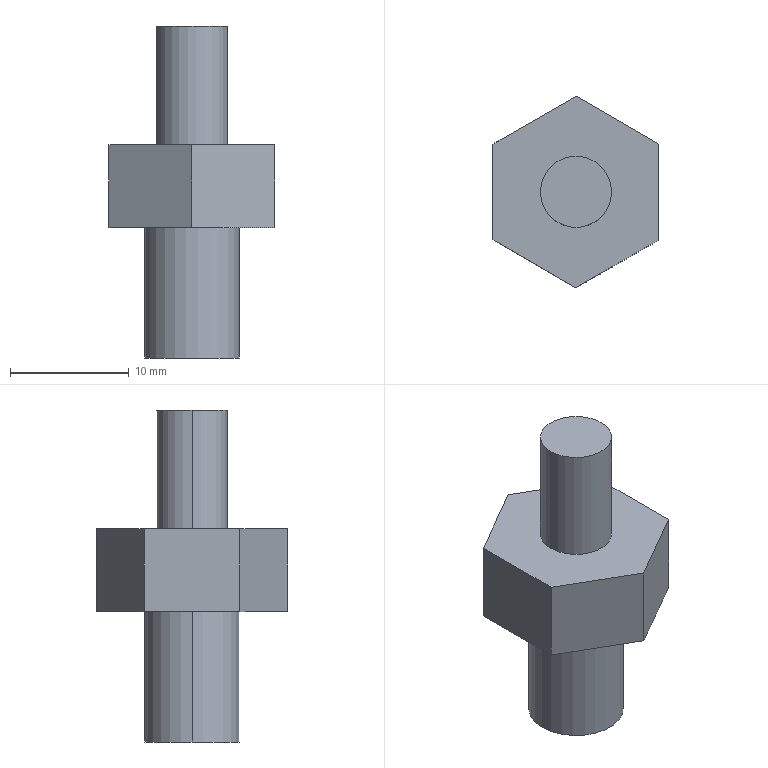Part | STEP file | Connecting bolt | 1 solid | 14 faces | box 14 x 16.166 x 28 mm | volume 2024 mm3 | plane 10 | cylinder 4 | commonest cylinder face diameters 6 x2 8 x2
STEP:
#1=CARTESIAN_POINT('',(-4.,0.,-14.5));
#2=VERTEX_POINT('',#1);
#3=CARTESIAN_POINT('',(4.,0.,-14.5));
#4=VERTEX_POINT('',#3);
#5=CARTESIAN_POINT('',(0.,0.,-14.5));
#6=DIRECTION('',(0.,0.,-1.));
#7=DIRECTION('',(-1.,0.,0.));
#8=AXIS2_PLACEMENT_3D('',#5,#6,#7);
#9=CIRCLE('',#8,4.);
#10=EDGE_CURVE('',#2,#4,#9,.T.);
#11=ORIENTED_EDGE('',*,*,#10,.F.);
#12=CARTESIAN_POINT('',(-4.,0.,-3.5));
#13=VERTEX_POINT('',#12);
#14=CARTESIAN_POINT('',(-4.,0.,-14.5));
#15=DIRECTION('',(0.,0.,1.));
#16=VECTOR('',#15,1000.);
#17=LINE('',#14,#16);
#18=EDGE_CURVE('',#2,#13,#17,.T.);
#19=ORIENTED_EDGE('',*,*,#18,.T.);
#20=CARTESIAN_POINT('',(4.,0.,-3.5));
#21=VERTEX_POINT('',#20);
#22=CARTESIAN_POINT('',(0.,0.,-3.5));
#23=DIRECTION('',(0.,0.,-1.));
#24=DIRECTION('',(1.,0.,0.));
#25=AXIS2_PLACEMENT_3D('',#22,#23,#24);
#26=CIRCLE('',#25,4.);
#27=EDGE_CURVE('',#13,#21,#26,.T.);
#28=ORIENTED_EDGE('',*,*,#27,.T.);
#29=CARTESIAN_POINT('',(4.,0.,-14.5));
#30=DIRECTION('',(0.,0.,1.));
#31=VECTOR('',#30,1000.);
#32=LINE('',#29,#31);
#33=EDGE_CURVE('',#4,#21,#32,.T.);
#34=ORIENTED_EDGE('',*,*,#33,.F.);
#35=EDGE_LOOP('',(#11,#19,#28,#34));
#36=FACE_OUTER_BOUND('',#35,.T.);
#37=CARTESIAN_POINT('',(0.,0.,-14.5));
#38=DIRECTION('',(0.,0.,1.));
#39=DIRECTION('',(1.,0.,0.));
#40=AXIS2_PLACEMENT_3D('',#37,#38,#39);
#41=CYLINDRICAL_SURFACE('',#40,4.);
#42=ADVANCED_FACE('',(#36),#41,.T.);
#43=CARTESIAN_POINT('',(3.,0.,13.5));
#44=VERTEX_POINT('',#43);
#45=CARTESIAN_POINT('',(-3.,0.,13.5));
#46=VERTEX_POINT('',#45);
#47=CARTESIAN_POINT('',(0.,0.,13.5));
#48=DIRECTION('',(0.,0.,1.));
#49=DIRECTION('',(1.,0.,0.));
#50=AXIS2_PLACEMENT_3D('',#47,#48,#49);
#51=CIRCLE('',#50,3.);
#52=EDGE_CURVE('',#44,#46,#51,.T.);
#53=ORIENTED_EDGE('',*,*,#52,.F.);
#54=CARTESIAN_POINT('',(3.,0.,3.5));
#55=VERTEX_POINT('',#54);
#56=CARTESIAN_POINT('',(3.,0.,13.5));
#57=DIRECTION('',(0.,0.,-1.));
#58=VECTOR('',#57,1000.);
#59=LINE('',#56,#58);
#60=EDGE_CURVE('',#44,#55,#59,.T.);
#61=ORIENTED_EDGE('',*,*,#60,.T.);
#62=CARTESIAN_POINT('',(-3.,0.,3.5));
#63=VERTEX_POINT('',#62);
#64=CARTESIAN_POINT('',(0.,0.,3.5));
#65=DIRECTION('',(0.,0.,1.));
#66=DIRECTION('',(1.,0.,0.));
#67=AXIS2_PLACEMENT_3D('',#64,#65,#66);
#68=CIRCLE('',#67,3.);
#69=EDGE_CURVE('',#55,#63,#68,.T.);
#70=ORIENTED_EDGE('',*,*,#69,.T.);
#71=CARTESIAN_POINT('',(-3.,0.,13.5));
#72=DIRECTION('',(0.,0.,-1.));
#73=VECTOR('',#72,1000.);
#74=LINE('',#71,#73);
#75=EDGE_CURVE('',#46,#63,#74,.T.);
#76=ORIENTED_EDGE('',*,*,#75,.F.);
#77=EDGE_LOOP('',(#53,#61,#70,#76));
#78=FACE_OUTER_BOUND('',#77,.T.);
#79=CARTESIAN_POINT('',(0.,0.,13.5));
#80=DIRECTION('',(0.,0.,-1.));
#81=DIRECTION('',(-1.,0.,0.));
#82=AXIS2_PLACEMENT_3D('',#79,#80,#81);
#83=CYLINDRICAL_SURFACE('',#82,3.);
#84=ADVANCED_FACE('',(#78),#83,.T.);
#85=CARTESIAN_POINT('',(-7.,-4.041,-3.5));
#86=VERTEX_POINT('',#85);
#87=CARTESIAN_POINT('',(0.,-8.083,-3.5));
#88=VERTEX_POINT('',#87);
#89=CARTESIAN_POINT('',(-7.,-4.041,-3.5));
#90=DIRECTION('',(0.866,-0.5,0.));
#91=VECTOR('',#90,1000.);
#92=LINE('',#89,#91);
#93=EDGE_CURVE('',#86,#88,#92,.T.);
#94=ORIENTED_EDGE('',*,*,#93,.F.);
#95=CARTESIAN_POINT('',(-7.,4.041,-3.5));
#96=VERTEX_POINT('',#95);
#97=CARTESIAN_POINT('',(-7.,4.041,-3.5));
#98=DIRECTION('',(0.,-1.,0.));
#99=VECTOR('',#98,1000.);
#100=LINE('',#97,#99);
#101=EDGE_CURVE('',#96,#86,#100,.T.);
#102=ORIENTED_EDGE('',*,*,#101,.F.);
#103=CARTESIAN_POINT('',(0.,8.083,-3.5));
#104=VERTEX_POINT('',#103);
#105=CARTESIAN_POINT('',(0.,8.083,-3.5));
#106=DIRECTION('',(-0.866,-0.5,0.));
#107=VECTOR('',#106,1000.);
#108=LINE('',#105,#107);
#109=EDGE_CURVE('',#104,#96,#108,.T.);
#110=ORIENTED_EDGE('',*,*,#109,.F.);
#111=CARTESIAN_POINT('',(7.,4.041,-3.5));
#112=VERTEX_POINT('',#111);
#113=CARTESIAN_POINT('',(7.,4.041,-3.5));
#114=DIRECTION('',(-0.866,0.5,0.));
#115=VECTOR('',#114,1000.);
#116=LINE('',#113,#115);
#117=EDGE_CURVE('',#112,#104,#116,.T.);
#118=ORIENTED_EDGE('',*,*,#117,.F.);
#119=CARTESIAN_POINT('',(7.,-4.041,-3.5));
#120=VERTEX_POINT('',#119);
#121=CARTESIAN_POINT('',(7.,-4.041,-3.5));
#122=DIRECTION('',(0.,1.,0.));
#123=VECTOR('',#122,1000.);
#124=LINE('',#121,#123);
#125=EDGE_CURVE('',#120,#112,#124,.T.);
#126=ORIENTED_EDGE('',*,*,#125,.F.);
#127=CARTESIAN_POINT('',(0.,-8.083,-3.5));
#128=DIRECTION('',(0.866,0.5,0.));
#129=VECTOR('',#128,1000.);
#130=LINE('',#127,#129);
#131=EDGE_CURVE('',#88,#120,#130,.T.);
#132=ORIENTED_EDGE('',*,*,#131,.F.);
#133=EDGE_LOOP('',(#94,#102,#110,#118,#126,#132));
#134=FACE_OUTER_BOUND('',#133,.T.);
#135=CARTESIAN_POINT('',(0.,0.,-3.5));
#136=DIRECTION('',(0.,0.,-1.));
#137=DIRECTION('',(1.,0.,0.));
#138=AXIS2_PLACEMENT_3D('',#135,#136,#137);
#139=CIRCLE('',#138,4.);
#140=EDGE_CURVE('',#21,#13,#139,.T.);
#141=ORIENTED_EDGE('',*,*,#140,.F.);
#142=ORIENTED_EDGE('',*,*,#27,.F.);
#143=EDGE_LOOP('',(#141,#142));
#144=FACE_BOUND('',#143,.T.);
#145=CARTESIAN_POINT('',(0.,0.,-3.5));
#146=DIRECTION('',(0.,0.,1.));
#147=DIRECTION('',(1.,0.,0.));
#148=AXIS2_PLACEMENT_3D('',#145,#146,#147);
#149=PLANE('',#148);
#150=ADVANCED_FACE('',(#134,#144),#149,.F.);
#151=CARTESIAN_POINT('',(-7.,-4.041,3.5));
#152=VERTEX_POINT('',#151);
#153=CARTESIAN_POINT('',(0.,-8.083,3.5));
#154=VERTEX_POINT('',#153);
#155=CARTESIAN_POINT('',(-7.,-4.041,3.5));
#156=DIRECTION('',(0.866,-0.5,0.));
#157=VECTOR('',#156,1000.);
#158=LINE('',#155,#157);
#159=EDGE_CURVE('',#152,#154,#158,.T.);
#160=ORIENTED_EDGE('',*,*,#159,.T.);
#161=CARTESIAN_POINT('',(7.,-4.041,3.5));
#162=VERTEX_POINT('',#161);
#163=CARTESIAN_POINT('',(0.,-8.083,3.5));
#164=DIRECTION('',(0.866,0.5,0.));
#165=VECTOR('',#164,1000.);
#166=LINE('',#163,#165);
#167=EDGE_CURVE('',#154,#162,#166,.T.);
#168=ORIENTED_EDGE('',*,*,#167,.T.);
#169=CARTESIAN_POINT('',(7.,4.041,3.5));
#170=VERTEX_POINT('',#169);
#171=CARTESIAN_POINT('',(7.,-4.041,3.5));
#172=DIRECTION('',(0.,1.,0.));
#173=VECTOR('',#172,1000.);
#174=LINE('',#171,#173);
#175=EDGE_CURVE('',#162,#170,#174,.T.);
#176=ORIENTED_EDGE('',*,*,#175,.T.);
#177=CARTESIAN_POINT('',(0.,8.083,3.5));
#178=VERTEX_POINT('',#177);
#179=CARTESIAN_POINT('',(7.,4.041,3.5));
#180=DIRECTION('',(-0.866,0.5,0.));
#181=VECTOR('',#180,1000.);
#182=LINE('',#179,#181);
#183=EDGE_CURVE('',#170,#178,#182,.T.);
#184=ORIENTED_EDGE('',*,*,#183,.T.);
#185=CARTESIAN_POINT('',(-7.,4.041,3.5));
#186=VERTEX_POINT('',#185);
#187=CARTESIAN_POINT('',(0.,8.083,3.5));
#188=DIRECTION('',(-0.866,-0.5,0.));
#189=VECTOR('',#188,1000.);
#190=LINE('',#187,#189);
#191=EDGE_CURVE('',#178,#186,#190,.T.);
#192=ORIENTED_EDGE('',*,*,#191,.T.);
#193=CARTESIAN_POINT('',(-7.,4.041,3.5));
#194=DIRECTION('',(0.,-1.,0.));
#195=VECTOR('',#194,1000.);
#196=LINE('',#193,#195);
#197=EDGE_CURVE('',#186,#152,#196,.T.);
#198=ORIENTED_EDGE('',*,*,#197,.T.);
#199=EDGE_LOOP('',(#160,#168,#176,#184,#192,#198));
#200=FACE_OUTER_BOUND('',#199,.T.);
#201=CARTESIAN_POINT('',(0.,0.,3.5));
#202=DIRECTION('',(0.,0.,1.));
#203=DIRECTION('',(1.,0.,0.));
#204=AXIS2_PLACEMENT_3D('',#201,#202,#203);
#205=CIRCLE('',#204,3.);
#206=EDGE_CURVE('',#63,#55,#205,.T.);
#207=ORIENTED_EDGE('',*,*,#206,.F.);
#208=ORIENTED_EDGE('',*,*,#69,.F.);
#209=EDGE_LOOP('',(#207,#208));
#210=FACE_BOUND('',#209,.T.);
#211=CARTESIAN_POINT('',(0.,0.,3.5));
#212=DIRECTION('',(0.,0.,1.));
#213=DIRECTION('',(1.,0.,0.));
#214=AXIS2_PLACEMENT_3D('',#211,#212,#213);
#215=PLANE('',#214);
#216=ADVANCED_FACE('',(#200,#210),#215,.T.);
#217=ORIENTED_EDGE('',*,*,#93,.T.);
#218=CARTESIAN_POINT('',(0.,-8.083,3.5));
#219=DIRECTION('',(0.,0.,-1.));
#220=VECTOR('',#219,1000.);
#221=LINE('',#218,#220);
#222=EDGE_CURVE('',#154,#88,#221,.T.);
#223=ORIENTED_EDGE('',*,*,#222,.F.);
#224=ORIENTED_EDGE('',*,*,#159,.F.);
#225=CARTESIAN_POINT('',(-7.,-4.041,3.5));
#226=DIRECTION('',(0.,0.,-1.));
#227=VECTOR('',#226,1000.);
#228=LINE('',#225,#227);
#229=EDGE_CURVE('',#152,#86,#228,.T.);
#230=ORIENTED_EDGE('',*,*,#229,.T.);
#231=EDGE_LOOP('',(#217,#223,#224,#230));
#232=FACE_OUTER_BOUND('',#231,.T.);
#233=CARTESIAN_POINT('',(-7.,-4.041,3.5));
#234=DIRECTION('',(0.5,0.866,0.));
#235=DIRECTION('',(-0.866,0.5,0.));
#236=AXIS2_PLACEMENT_3D('',#233,#234,#235);
#237=PLANE('',#236);
#238=ADVANCED_FACE('',(#232),#237,.F.);
#239=ORIENTED_EDGE('',*,*,#131,.T.);
#240=CARTESIAN_POINT('',(7.,-4.041,3.5));
#241=DIRECTION('',(0.,0.,-1.));
#242=VECTOR('',#241,1000.);
#243=LINE('',#240,#242);
#244=EDGE_CURVE('',#162,#120,#243,.T.);
#245=ORIENTED_EDGE('',*,*,#244,.F.);
#246=ORIENTED_EDGE('',*,*,#167,.F.);
#247=ORIENTED_EDGE('',*,*,#222,.T.);
#248=EDGE_LOOP('',(#239,#245,#246,#247));
#249=FACE_OUTER_BOUND('',#248,.T.);
#250=CARTESIAN_POINT('',(0.,-8.083,3.5));
#251=DIRECTION('',(-0.5,0.866,0.));
#252=DIRECTION('',(-0.866,-0.5,0.));
#253=AXIS2_PLACEMENT_3D('',#250,#251,#252);
#254=PLANE('',#253);
#255=ADVANCED_FACE('',(#249),#254,.F.);
#256=ORIENTED_EDGE('',*,*,#125,.T.);
#257=CARTESIAN_POINT('',(7.,4.041,3.5));
#258=DIRECTION('',(0.,0.,-1.));
#259=VECTOR('',#258,1000.);
#260=LINE('',#257,#259);
#261=EDGE_CURVE('',#170,#112,#260,.T.);
#262=ORIENTED_EDGE('',*,*,#261,.F.);
#263=ORIENTED_EDGE('',*,*,#175,.F.);
#264=ORIENTED_EDGE('',*,*,#244,.T.);
#265=EDGE_LOOP('',(#256,#262,#263,#264));
#266=FACE_OUTER_BOUND('',#265,.T.);
#267=CARTESIAN_POINT('',(7.,-4.041,3.5));
#268=DIRECTION('',(-1.,0.,0.));
#269=DIRECTION('',(0.,-1.,0.));
#270=AXIS2_PLACEMENT_3D('',#267,#268,#269);
#271=PLANE('',#270);
#272=ADVANCED_FACE('',(#266),#271,.F.);
#273=ORIENTED_EDGE('',*,*,#117,.T.);
#274=CARTESIAN_POINT('',(0.,8.083,3.5));
#275=DIRECTION('',(0.,0.,-1.));
#276=VECTOR('',#275,1000.);
#277=LINE('',#274,#276);
#278=EDGE_CURVE('',#178,#104,#277,.T.);
#279=ORIENTED_EDGE('',*,*,#278,.F.);
#280=ORIENTED_EDGE('',*,*,#183,.F.);
#281=ORIENTED_EDGE('',*,*,#261,.T.);
#282=EDGE_LOOP('',(#273,#279,#280,#281));
#283=FACE_OUTER_BOUND('',#282,.T.);
#284=CARTESIAN_POINT('',(7.,4.041,3.5));
#285=DIRECTION('',(-0.5,-0.866,0.));
#286=DIRECTION('',(0.866,-0.5,0.));
#287=AXIS2_PLACEMENT_3D('',#284,#285,#286);
#288=PLANE('',#287);
#289=ADVANCED_FACE('',(#283),#288,.F.);
#290=ORIENTED_EDGE('',*,*,#109,.T.);
#291=CARTESIAN_POINT('',(-7.,4.041,3.5));
#292=DIRECTION('',(0.,0.,-1.));
#293=VECTOR('',#292,1000.);
#294=LINE('',#291,#293);
#295=EDGE_CURVE('',#186,#96,#294,.T.);
#296=ORIENTED_EDGE('',*,*,#295,.F.);
#297=ORIENTED_EDGE('',*,*,#191,.F.);
#298=ORIENTED_EDGE('',*,*,#278,.T.);
#299=EDGE_LOOP('',(#290,#296,#297,#298));
#300=FACE_OUTER_BOUND('',#299,.T.);
#301=CARTESIAN_POINT('',(0.,8.083,3.5));
#302=DIRECTION('',(0.5,-0.866,0.));
#303=DIRECTION('',(0.866,0.5,0.));
#304=AXIS2_PLACEMENT_3D('',#301,#302,#303);
#305=PLANE('',#304);
#306=ADVANCED_FACE('',(#300),#305,.F.);
#307=ORIENTED_EDGE('',*,*,#101,.T.);
#308=ORIENTED_EDGE('',*,*,#229,.F.);
#309=ORIENTED_EDGE('',*,*,#197,.F.);
#310=ORIENTED_EDGE('',*,*,#295,.T.);
#311=EDGE_LOOP('',(#307,#308,#309,#310));
#312=FACE_OUTER_BOUND('',#311,.T.);
#313=CARTESIAN_POINT('',(-7.,4.041,3.5));
#314=DIRECTION('',(1.,0.,0.));
#315=DIRECTION('',(0.,1.,0.));
#316=AXIS2_PLACEMENT_3D('',#313,#314,#315);
#317=PLANE('',#316);
#318=ADVANCED_FACE('',(#312),#317,.F.);
#319=ORIENTED_EDGE('',*,*,#60,.F.);
#320=CARTESIAN_POINT('',(0.,0.,13.5));
#321=DIRECTION('',(0.,0.,1.));
#322=DIRECTION('',(1.,0.,0.));
#323=AXIS2_PLACEMENT_3D('',#320,#321,#322);
#324=CIRCLE('',#323,3.);
#325=EDGE_CURVE('',#46,#44,#324,.T.);
#326=ORIENTED_EDGE('',*,*,#325,.F.);
#327=ORIENTED_EDGE('',*,*,#75,.T.);
#328=ORIENTED_EDGE('',*,*,#206,.T.);
#329=EDGE_LOOP('',(#319,#326,#327,#328));
#330=FACE_OUTER_BOUND('',#329,.T.);
#331=CARTESIAN_POINT('',(0.,0.,13.5));
#332=DIRECTION('',(0.,0.,-1.));
#333=DIRECTION('',(-1.,0.,0.));
#334=AXIS2_PLACEMENT_3D('',#331,#332,#333);
#335=CYLINDRICAL_SURFACE('',#334,3.);
#336=ADVANCED_FACE('',(#330),#335,.T.);
#337=ORIENTED_EDGE('',*,*,#325,.T.);
#338=ORIENTED_EDGE('',*,*,#52,.T.);
#339=EDGE_LOOP('',(#337,#338));
#340=FACE_OUTER_BOUND('',#339,.T.);
#341=CARTESIAN_POINT('',(0.,0.,13.5));
#342=DIRECTION('',(0.,0.,1.));
#343=DIRECTION('',(1.,0.,0.));
#344=AXIS2_PLACEMENT_3D('',#341,#342,#343);
#345=PLANE('',#344);
#346=ADVANCED_FACE('',(#340),#345,.T.);
#347=ORIENTED_EDGE('',*,*,#18,.F.);
#348=CARTESIAN_POINT('',(0.,0.,-14.5));
#349=DIRECTION('',(0.,0.,-1.));
#350=DIRECTION('',(-1.,0.,0.));
#351=AXIS2_PLACEMENT_3D('',#348,#349,#350);
#352=CIRCLE('',#351,4.);
#353=EDGE_CURVE('',#4,#2,#352,.T.);
#354=ORIENTED_EDGE('',*,*,#353,.F.);
#355=ORIENTED_EDGE('',*,*,#33,.T.);
#356=ORIENTED_EDGE('',*,*,#140,.T.);
#357=EDGE_LOOP('',(#347,#354,#355,#356));
#358=FACE_OUTER_BOUND('',#357,.T.);
#359=CARTESIAN_POINT('',(0.,0.,-14.5));
#360=DIRECTION('',(0.,0.,1.));
#361=DIRECTION('',(1.,0.,0.));
#362=AXIS2_PLACEMENT_3D('',#359,#360,#361);
#363=CYLINDRICAL_SURFACE('',#362,4.);
#364=ADVANCED_FACE('',(#358),#363,.T.);
#365=ORIENTED_EDGE('',*,*,#353,.T.);
#366=ORIENTED_EDGE('',*,*,#10,.T.);
#367=EDGE_LOOP('',(#365,#366));
#368=FACE_OUTER_BOUND('',#367,.T.);
#369=CARTESIAN_POINT('',(0.,0.,-14.5));
#370=DIRECTION('',(0.,0.,-1.));
#371=DIRECTION('',(-1.,0.,0.));
#372=AXIS2_PLACEMENT_3D('',#369,#370,#371);
#373=PLANE('',#372);
#374=ADVANCED_FACE('',(#368),#373,.T.);
#375=CLOSED_SHELL('',(#42,#84,#150,#216,#238,#255,#272,#289,#306,#318,#336,#346,#364,#374));
#376=MANIFOLD_SOLID_BREP('',#375);
#377=CARTESIAN_POINT('',(0.,0.,0.));
#378=DIRECTION('',(0.,0.,1.));
#379=DIRECTION('',(1.,0.,0.));
#380=AXIS2_PLACEMENT_3D('',#377,#378,#379);
#381=(LENGTH_UNIT()NAMED_UNIT(*)SI_UNIT(.MILLI.,.METRE.));
#382=UNCERTAINTY_MEASURE_WITH_UNIT(LENGTH_MEASURE(0.00001),#381,'','');
#383=(NAMED_UNIT(*)PLANE_ANGLE_UNIT()SI_UNIT($,.RADIAN.));
#384=(NAMED_UNIT(*)SI_UNIT($,.STERADIAN.)SOLID_ANGLE_UNIT());
#385=(GEOMETRIC_REPRESENTATION_CONTEXT(3)GLOBAL_UNCERTAINTY_ASSIGNED_CONTEXT((#382))GLOBAL_UNIT_ASSIGNED_CONTEXT((#381,#383,#384))REPRESENTATION_CONTEXT('',''));
#386=ADVANCED_BREP_SHAPE_REPRESENTATION('',(#376,#380),#385);